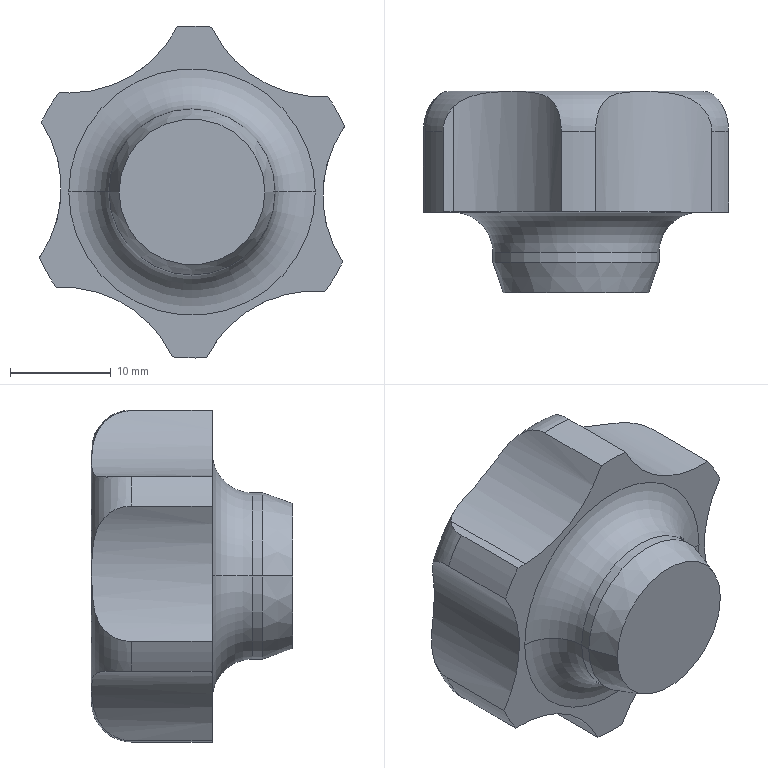Part | STEP file | Boom Knob Head | 1 solid | 40 faces | box 30.33 x 20 x 33 mm | volume 9480 mm3 | cylinder 17 | torus 14 | plane 7 | cone 2 | commonest cylinder face diameters 24 x7 33 x6 16.5 x2 20 x2